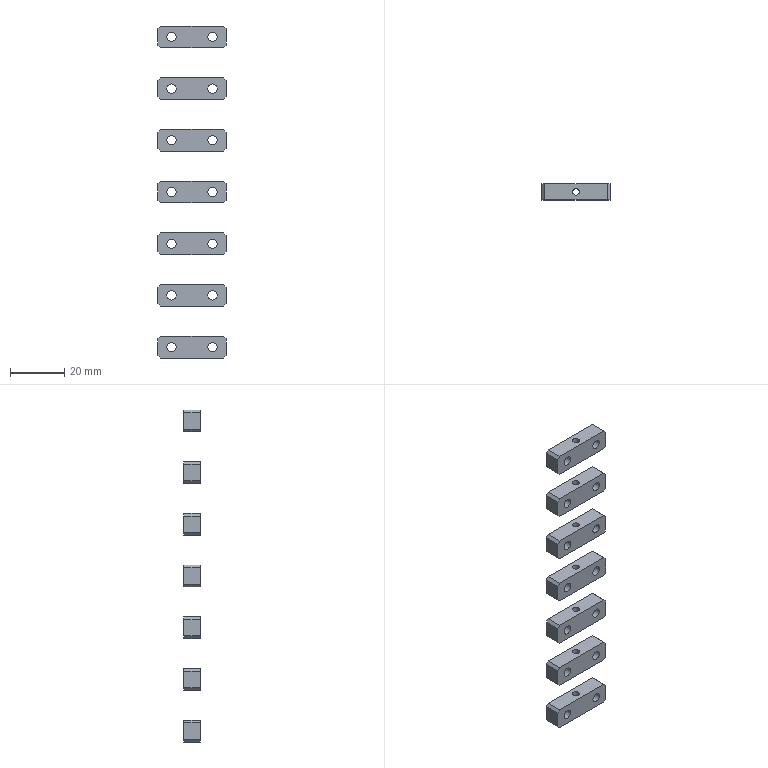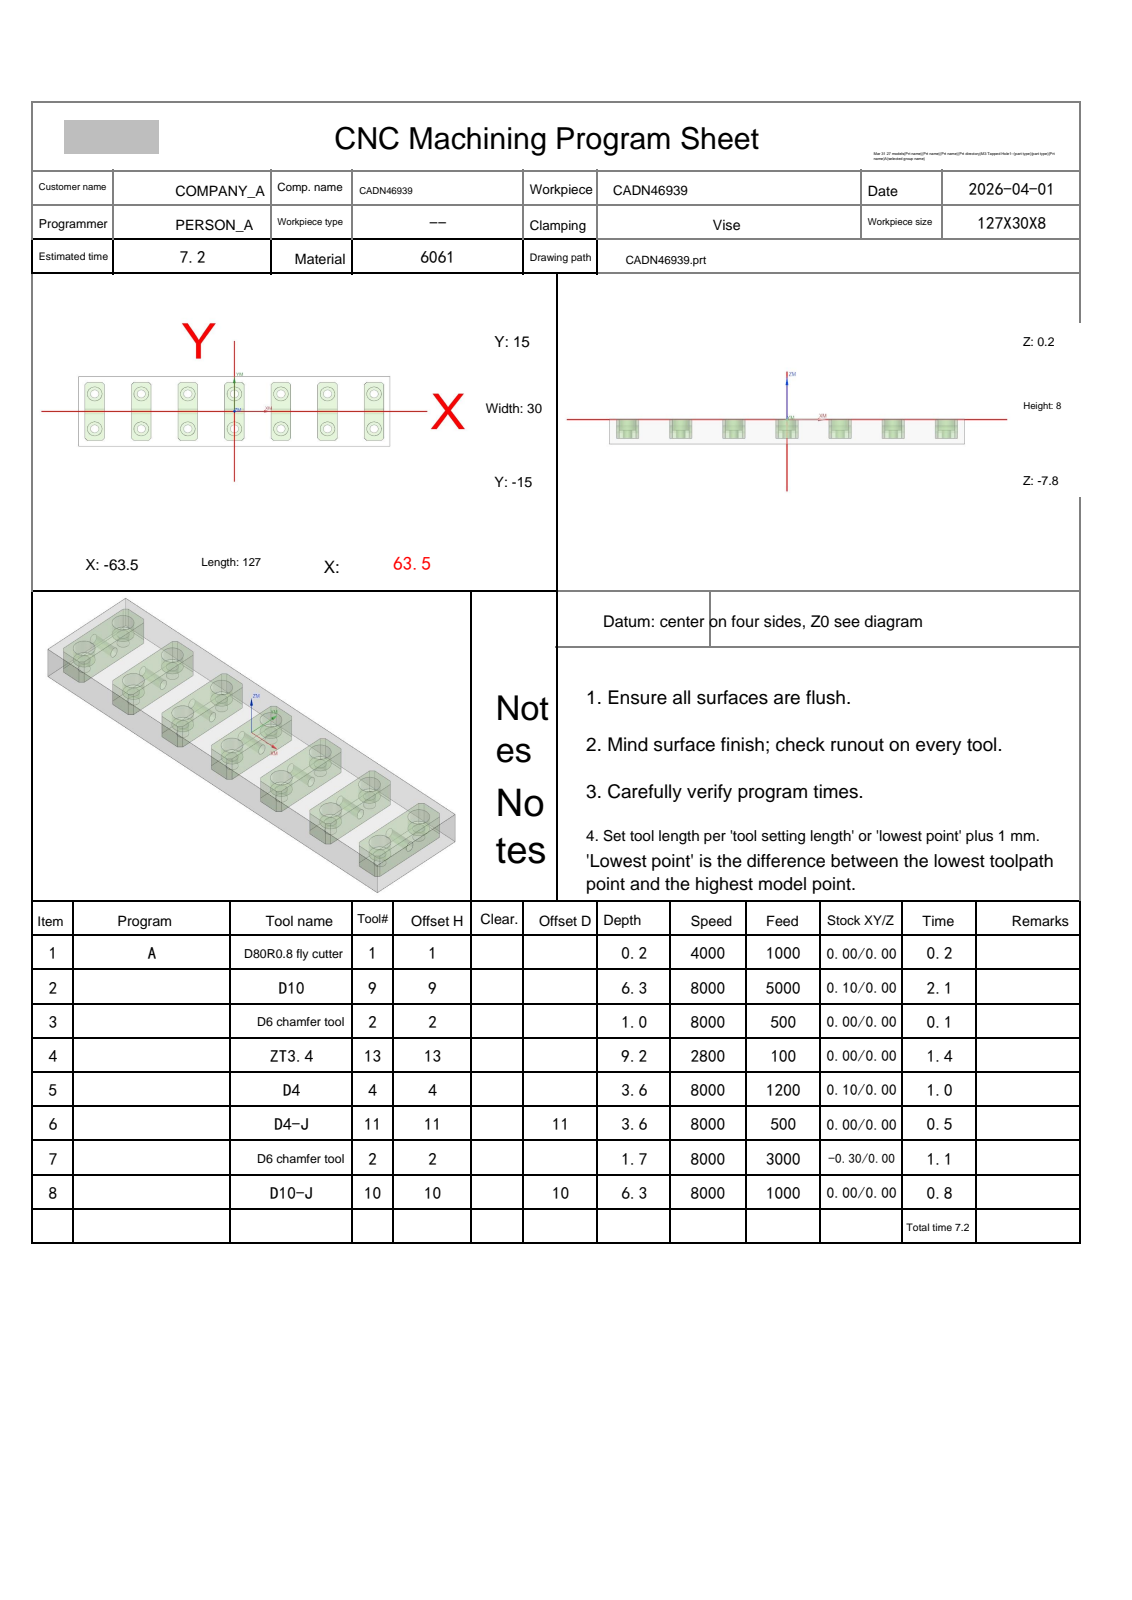NC program | NX | posted by the shop | part box 25 x 6 x 122 mm
Lines 1 to 33 of 3537:
%
O0001
(Machine time: 8.64 MIN)
(===Total Tool:7===)
(T1=D80R0.8 fly cutter D=80.  R=0.8  D-  H01 Z=0.    )
(T9=D10     D=10.  R=0.   D-  H09 Z=-6.1  )
(T2=D6 chamfer tool   D=6.   R=0.   D-  H02 Z=-1.5  )
(T13=ZT3.4  D=3.4  DR_a=118 D-  H13 Z=-9.02 )
(T4=D4      D=4.   R=0.   D-  H04 Z=-3.4  )
(T11=D4-J   D=4.   R=0.   D11 H11 Z=-3.4  )
(T10=D10-J  D=10.  R=0.   D10 H10 Z=-6.1  )
G80 G90 G17 G49 G40
G91 G28 Z0
M01
N1 T01 M06
(D80R0.8 fly cutter  D=80. R=0.8 H=01 ce=0.00 di=0.00)
G00 G90 G54 X106. Y0.0 M03 S4000
G43 H01 Z20.
M08
Z2.
G01 Z0.0 F1000.
X101.
X-101.
X-106.
Z2.
G00 Z20.
G91 G28 Z0.0
M05
M09
G91 G28 Z0.0
M01